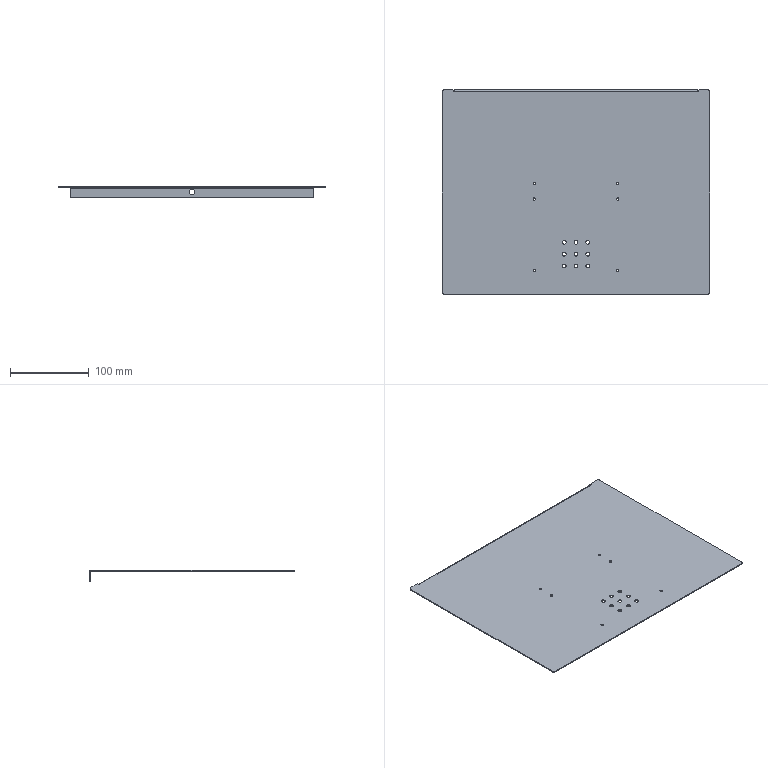Part | SolidWorks | features ICE 2, EdgeFlange 1, FlatPattern 1, SMBaseFlange 1, SheetMetal 1 | 1 solid | 62 faces | box 340 x 260 x 15 mm | volume 110561 mm3 | cylinder 38 | plane 24 | commonest cylinder face diameters 5 x18 3 x13 5.4 x5 7 x2